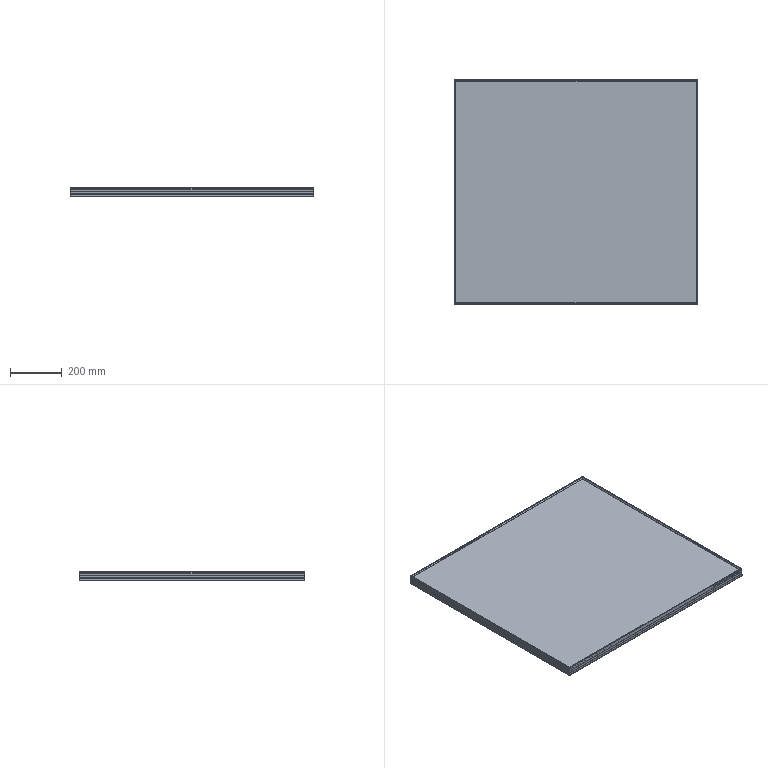Part | 6 solids | 202 faces | box 940 x 870 x 36 mm | volume 3581114 mm3 | plane 148 | cylinder 54 | commonest cylinder face diameters 7 x50 5 x4